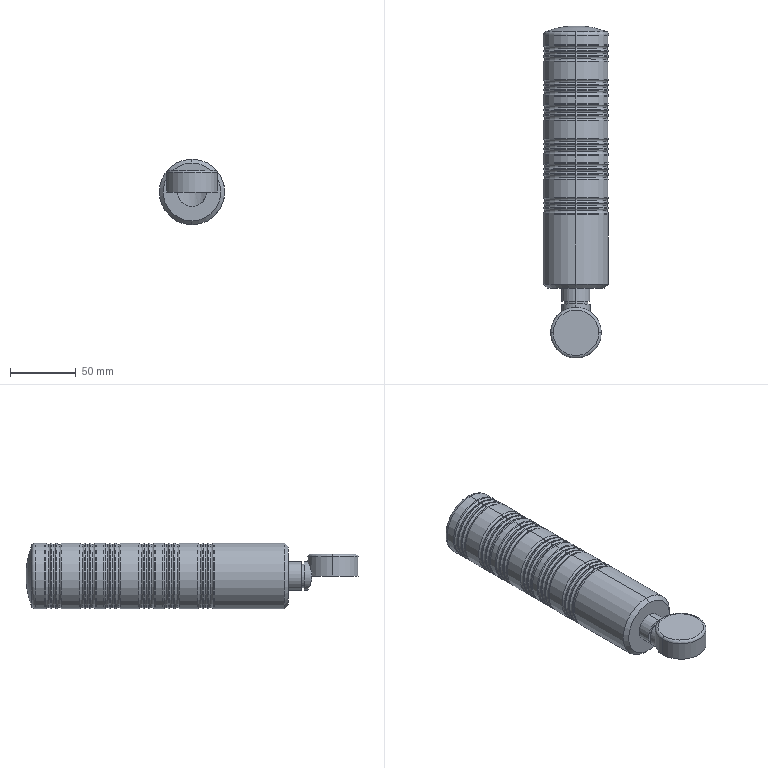Part | SolidWorks | features ICE 9, Fillet 2, LPattern 2, Chamfer 1, Dome 1, Extrusion 1, RevCut 1 | 7 solids | 161 faces | box 50 x 253.304 x 50 mm | volume 205470 mm3 | torus 76 | cylinder 65 | plane 17 | cone 2 | sphere 1 | commonest cylinder face diameters 50 x50 46 x6 38.7 x3 18 x2 21.5 x2 21.9 x2